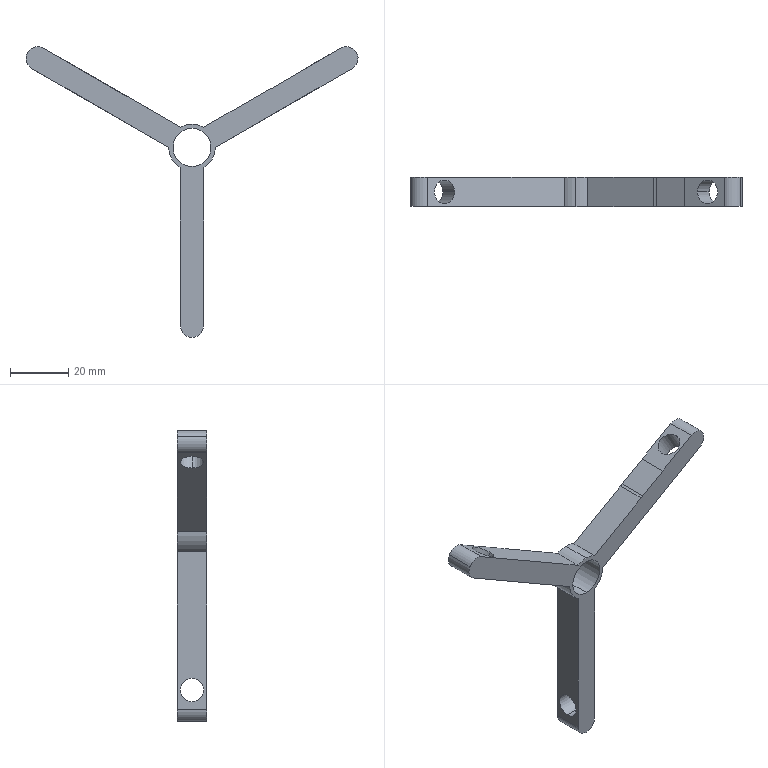Part | SolidWorks | features CirPattern 2, Fillet 2, ICE 2, Cut 1, Extrusion 1 | 1 solid | 29 faces | box 113.655 x 10 x 99.5 mm | volume 13029 mm3 | cylinder 19 | plane 10 | commonest cylinder face diameters 8 x12 16 x4 13 x2 10 x1
STEP:
#1=CARTESIAN_POINT('',(48.481,5.,32.609));
#2=VERTEX_POINT('',#1);
#3=CARTESIAN_POINT('',(41.552,5.,28.609));
#4=VERTEX_POINT('',#3);
#5=CARTESIAN_POINT('',(45.017,5.,30.609));
#6=DIRECTION('',(0.5,0.,-0.866));
#7=DIRECTION('',(-0.866,0.,-0.5));
#8=AXIS2_PLACEMENT_3D('',#5,#6,#7);
#9=CIRCLE('',#8,4.);
#10=EDGE_CURVE('',#2,#4,#9,.T.);
#11=ORIENTED_EDGE('',*,*,#10,.F.);
#12=CARTESIAN_POINT('',(52.481,5.,25.681));
#13=VERTEX_POINT('',#12);
#14=CARTESIAN_POINT('',(44.981,5.,38.671));
#15=DIRECTION('',(0.5,0.,-0.866));
#16=VECTOR('',#15,1000.);
#17=LINE('',#14,#16);
#18=EDGE_CURVE('',#2,#13,#17,.T.);
#19=ORIENTED_EDGE('',*,*,#18,.T.);
#20=CARTESIAN_POINT('',(45.552,5.,21.681));
#21=VERTEX_POINT('',#20);
#22=CARTESIAN_POINT('',(49.017,5.,23.681));
#23=DIRECTION('',(0.5,0.,-0.866));
#24=DIRECTION('',(-0.866,0.,-0.5));
#25=AXIS2_PLACEMENT_3D('',#22,#23,#24);
#26=CIRCLE('',#25,4.);
#27=EDGE_CURVE('',#13,#21,#26,.T.);
#28=ORIENTED_EDGE('',*,*,#27,.T.);
#29=CARTESIAN_POINT('',(38.052,5.,34.671));
#30=DIRECTION('',(0.5,0.,-0.866));
#31=VECTOR('',#30,1000.);
#32=LINE('',#29,#31);
#33=EDGE_CURVE('',#4,#21,#32,.T.);
#34=ORIENTED_EDGE('',*,*,#33,.F.);
#35=EDGE_LOOP('',(#11,#19,#28,#34));
#36=FACE_OUTER_BOUND('',#35,.T.);
#37=CARTESIAN_POINT('',(41.517,5.,36.671));
#38=DIRECTION('',(0.5,0.,-0.866));
#39=DIRECTION('',(-0.866,0.,-0.5));
#40=AXIS2_PLACEMENT_3D('',#37,#38,#39);
#41=CYLINDRICAL_SURFACE('',#40,4.);
#42=ADVANCED_FACE('',(#36),#41,.F.);
#43=CARTESIAN_POINT('',(-52.481,5.,25.681));
#44=VERTEX_POINT('',#43);
#45=CARTESIAN_POINT('',(-45.552,5.,21.681));
#46=VERTEX_POINT('',#45);
#47=CARTESIAN_POINT('',(-49.017,5.,23.681));
#48=DIRECTION('',(0.5,0.,0.866));
#49=DIRECTION('',(0.866,0.,-0.5));
#50=AXIS2_PLACEMENT_3D('',#47,#48,#49);
#51=CIRCLE('',#50,4.);
#52=EDGE_CURVE('',#44,#46,#51,.T.);
#53=ORIENTED_EDGE('',*,*,#52,.F.);
#54=CARTESIAN_POINT('',(-48.481,5.,32.609));
#55=VERTEX_POINT('',#54);
#56=CARTESIAN_POINT('',(-55.981,5.,19.619));
#57=DIRECTION('',(0.5,0.,0.866));
#58=VECTOR('',#57,1000.);
#59=LINE('',#56,#58);
#60=EDGE_CURVE('',#44,#55,#59,.T.);
#61=ORIENTED_EDGE('',*,*,#60,.T.);
#62=CARTESIAN_POINT('',(-41.552,5.,28.609));
#63=VERTEX_POINT('',#62);
#64=CARTESIAN_POINT('',(-45.017,5.,30.609));
#65=DIRECTION('',(0.5,0.,0.866));
#66=DIRECTION('',(0.866,0.,-0.5));
#67=AXIS2_PLACEMENT_3D('',#64,#65,#66);
#68=CIRCLE('',#67,4.);
#69=EDGE_CURVE('',#55,#63,#68,.T.);
#70=ORIENTED_EDGE('',*,*,#69,.T.);
#71=CARTESIAN_POINT('',(-49.052,5.,15.619));
#72=DIRECTION('',(0.5,0.,0.866));
#73=VECTOR('',#72,1000.);
#74=LINE('',#71,#73);
#75=EDGE_CURVE('',#46,#63,#74,.T.);
#76=ORIENTED_EDGE('',*,*,#75,.F.);
#77=EDGE_LOOP('',(#53,#61,#70,#76));
#78=FACE_OUTER_BOUND('',#77,.T.);
#79=CARTESIAN_POINT('',(-52.517,5.,17.619));
#80=DIRECTION('',(0.5,0.,0.866));
#81=DIRECTION('',(0.866,0.,-0.5));
#82=AXIS2_PLACEMENT_3D('',#79,#80,#81);
#83=CYLINDRICAL_SURFACE('',#82,4.);
#84=ADVANCED_FACE('',(#78),#83,.F.);
#85=CARTESIAN_POINT('',(4.,5.,-58.29));
#86=VERTEX_POINT('',#85);
#87=CARTESIAN_POINT('',(4.,5.,-50.29));
#88=VERTEX_POINT('',#87);
#89=CARTESIAN_POINT('',(4.,5.,-54.29));
#90=DIRECTION('',(-1.,0.,0.));
#91=DIRECTION('',(0.,0.,1.));
#92=AXIS2_PLACEMENT_3D('',#89,#90,#91);
#93=CIRCLE('',#92,4.);
#94=EDGE_CURVE('',#86,#88,#93,.T.);
#95=ORIENTED_EDGE('',*,*,#94,.F.);
#96=CARTESIAN_POINT('',(-4.,5.,-58.29));
#97=VERTEX_POINT('',#96);
#98=CARTESIAN_POINT('',(11.,5.,-58.29));
#99=DIRECTION('',(-1.,0.,0.));
#100=VECTOR('',#99,1000.);
#101=LINE('',#98,#100);
#102=EDGE_CURVE('',#86,#97,#101,.T.);
#103=ORIENTED_EDGE('',*,*,#102,.T.);
#104=CARTESIAN_POINT('',(-4.,5.,-50.29));
#105=VERTEX_POINT('',#104);
#106=CARTESIAN_POINT('',(-4.,5.,-54.29));
#107=DIRECTION('',(-1.,0.,0.));
#108=DIRECTION('',(0.,0.,1.));
#109=AXIS2_PLACEMENT_3D('',#106,#107,#108);
#110=CIRCLE('',#109,4.);
#111=EDGE_CURVE('',#97,#105,#110,.T.);
#112=ORIENTED_EDGE('',*,*,#111,.T.);
#113=CARTESIAN_POINT('',(11.,5.,-50.29));
#114=DIRECTION('',(-1.,0.,0.));
#115=VECTOR('',#114,1000.);
#116=LINE('',#113,#115);
#117=EDGE_CURVE('',#88,#105,#116,.T.);
#118=ORIENTED_EDGE('',*,*,#117,.F.);
#119=EDGE_LOOP('',(#95,#103,#112,#118));
#120=FACE_OUTER_BOUND('',#119,.T.);
#121=CARTESIAN_POINT('',(11.,5.,-54.29));
#122=DIRECTION('',(-1.,0.,0.));
#123=DIRECTION('',(0.,0.,1.));
#124=AXIS2_PLACEMENT_3D('',#121,#122,#123);
#125=CYLINDRICAL_SURFACE('',#124,4.);
#126=ADVANCED_FACE('',(#120),#125,.F.);
#127=CARTESIAN_POINT('',(0.,0.,8.));
#128=VERTEX_POINT('',#127);
#129=CARTESIAN_POINT('',(-4.,0.,6.928));
#130=VERTEX_POINT('',#129);
#131=CARTESIAN_POINT('',(0.,0.,0.));
#132=DIRECTION('',(0.,-1.,0.));
#133=DIRECTION('',(0.,0.,1.));
#134=AXIS2_PLACEMENT_3D('',#131,#132,#133);
#135=CIRCLE('',#134,8.);
#136=EDGE_CURVE('',#128,#130,#135,.T.);
#137=ORIENTED_EDGE('',*,*,#136,.F.);
#138=CARTESIAN_POINT('',(0.,10.,8.));
#139=VERTEX_POINT('',#138);
#140=CARTESIAN_POINT('',(0.,-14.,8.));
#141=DIRECTION('',(0.,1.,0.));
#142=VECTOR('',#141,1000.);
#143=LINE('',#140,#142);
#144=EDGE_CURVE('',#128,#139,#143,.T.);
#145=ORIENTED_EDGE('',*,*,#144,.T.);
#146=CARTESIAN_POINT('',(-4.,10.,6.928));
#147=VERTEX_POINT('',#146);
#148=CARTESIAN_POINT('',(0.,10.,0.));
#149=DIRECTION('',(0.,-1.,0.));
#150=DIRECTION('',(-0.866,0.,-0.5));
#151=AXIS2_PLACEMENT_3D('',#148,#149,#150);
#152=CIRCLE('',#151,8.);
#153=EDGE_CURVE('',#139,#147,#152,.T.);
#154=ORIENTED_EDGE('',*,*,#153,.T.);
#155=CARTESIAN_POINT('',(-4.,-14.,6.928));
#156=DIRECTION('',(0.,1.,0.));
#157=VECTOR('',#156,1000.);
#158=LINE('',#155,#157);
#159=EDGE_CURVE('',#130,#147,#158,.T.);
#160=ORIENTED_EDGE('',*,*,#159,.F.);
#161=EDGE_LOOP('',(#137,#145,#154,#160));
#162=FACE_OUTER_BOUND('',#161,.T.);
#163=CARTESIAN_POINT('',(0.,-14.,0.));
#164=DIRECTION('',(0.,1.,0.));
#165=DIRECTION('',(0.,0.,1.));
#166=AXIS2_PLACEMENT_3D('',#163,#164,#165);
#167=CYLINDRICAL_SURFACE('',#166,8.);
#168=ADVANCED_FACE('',(#162),#167,.T.);
#169=CARTESIAN_POINT('',(0.,10.,6.5));
#170=VERTEX_POINT('',#169);
#171=CARTESIAN_POINT('',(0.,10.,-6.5));
#172=VERTEX_POINT('',#171);
#173=CARTESIAN_POINT('',(0.,10.,0.));
#174=DIRECTION('',(0.,-1.,0.));
#175=DIRECTION('',(0.,0.,-1.));
#176=AXIS2_PLACEMENT_3D('',#173,#174,#175);
#177=CIRCLE('',#176,6.5);
#178=EDGE_CURVE('',#170,#172,#177,.T.);
#179=ORIENTED_EDGE('',*,*,#178,.F.);
#180=CARTESIAN_POINT('',(0.,0.,6.5));
#181=VERTEX_POINT('',#180);
#182=CARTESIAN_POINT('',(0.,10.,6.5));
#183=DIRECTION('',(0.,-1.,0.));
#184=VECTOR('',#183,1000.);
#185=LINE('',#182,#184);
#186=EDGE_CURVE('',#170,#181,#185,.T.);
#187=ORIENTED_EDGE('',*,*,#186,.T.);
#188=CARTESIAN_POINT('',(0.,0.,-6.5));
#189=VERTEX_POINT('',#188);
#190=CARTESIAN_POINT('',(0.,0.,0.));
#191=DIRECTION('',(0.,-1.,0.));
#192=DIRECTION('',(0.,0.,-1.));
#193=AXIS2_PLACEMENT_3D('',#190,#191,#192);
#194=CIRCLE('',#193,6.5);
#195=EDGE_CURVE('',#181,#189,#194,.T.);
#196=ORIENTED_EDGE('',*,*,#195,.T.);
#197=CARTESIAN_POINT('',(0.,10.,-6.5));
#198=DIRECTION('',(0.,-1.,0.));
#199=VECTOR('',#198,1000.);
#200=LINE('',#197,#199);
#201=EDGE_CURVE('',#172,#189,#200,.T.);
#202=ORIENTED_EDGE('',*,*,#201,.F.);
#203=EDGE_LOOP('',(#179,#187,#196,#202));
#204=FACE_OUTER_BOUND('',#203,.T.);
#205=CARTESIAN_POINT('',(0.,10.,0.));
#206=DIRECTION('',(0.,-1.,0.));
#207=DIRECTION('',(0.,0.,-1.));
#208=AXIS2_PLACEMENT_3D('',#205,#206,#207);
#209=CYLINDRICAL_SURFACE('',#208,6.5);
#210=ADVANCED_FACE('',(#204),#209,.F.);
#211=CARTESIAN_POINT('',(27.386,10.,20.333));
#212=VERTEX_POINT('',#211);
#213=CARTESIAN_POINT('',(36.971,10.,25.964));
#214=VERTEX_POINT('',#213);
#215=CARTESIAN_POINT('',(36.971,10.,25.964));
#216=DIRECTION('',(0.8622,0.,0.5066));
#217=VECTOR('',#216,1000.);
#218=LINE('',#215,#217);
#219=EDGE_CURVE('',#212,#214,#218,.T.);
#220=ORIENTED_EDGE('',*,*,#219,.F.);
#221=CARTESIAN_POINT('',(27.386,0.,20.333));
#222=VERTEX_POINT('',#221);
#223=CARTESIAN_POINT('',(27.386,0.,20.333));
#224=DIRECTION('',(0.,-1.,0.));
#225=VECTOR('',#224,1000.);
#226=LINE('',#223,#225);
#227=EDGE_CURVE('',#212,#222,#226,.T.);
#228=ORIENTED_EDGE('',*,*,#227,.T.);
#229=CARTESIAN_POINT('',(36.971,0.,25.964));
#230=VERTEX_POINT('',#229);
#231=CARTESIAN_POINT('',(36.971,0.,25.964));
#232=DIRECTION('',(0.8622,0.,0.5066));
#233=VECTOR('',#232,1000.);
#234=LINE('',#231,#233);
#235=EDGE_CURVE('',#222,#230,#234,.T.);
#236=ORIENTED_EDGE('',*,*,#235,.T.);
#237=CARTESIAN_POINT('',(36.971,10.,25.964));
#238=DIRECTION('',(0.,-1.,0.));
#239=VECTOR('',#238,1000.);
#240=LINE('',#237,#239);
#241=EDGE_CURVE('',#214,#230,#240,.T.);
#242=ORIENTED_EDGE('',*,*,#241,.F.);
#243=EDGE_LOOP('',(#220,#228,#236,#242));
#244=FACE_OUTER_BOUND('',#243,.T.);
#245=CARTESIAN_POINT('',(36.971,10.,25.964));
#246=DIRECTION('',(0.5066,0.,-0.8622));
#247=DIRECTION('',(-0.8622,0.,-0.5066));
#248=AXIS2_PLACEMENT_3D('',#245,#246,#247);
#249=PLANE('',#248);
#250=ADVANCED_FACE('',(#244),#249,.F.);
#251=CARTESIAN_POINT('',(45.017,5.,30.609));
#252=DIRECTION('',(0.5,0.,-0.866));
#253=DIRECTION('',(-0.866,0.,-0.5));
#254=AXIS2_PLACEMENT_3D('',#251,#252,#253);
#255=CIRCLE('',#254,4.);
#256=EDGE_CURVE('',#4,#2,#255,.T.);
#257=ORIENTED_EDGE('',*,*,#256,.T.);
#258=ORIENTED_EDGE('',*,*,#10,.T.);
#259=EDGE_LOOP('',(#257,#258));
#260=FACE_BOUND('',#259,.T.);
#261=CARTESIAN_POINT('',(50.828,0.,33.964));
#262=VERTEX_POINT('',#261);
#263=CARTESIAN_POINT('',(54.292,0.,35.964));
#264=DIRECTION('',(0.866,0.,0.5));
#265=VECTOR('',#264,1000.);
#266=LINE('',#263,#265);
#267=EDGE_CURVE('',#230,#262,#266,.T.);
#268=ORIENTED_EDGE('',*,*,#267,.T.);
#269=CARTESIAN_POINT('',(50.828,10.,33.964));
#270=VERTEX_POINT('',#269);
#271=CARTESIAN_POINT('',(50.828,10.,33.964));
#272=DIRECTION('',(0.,1.,0.));
#273=VECTOR('',#272,1000.);
#274=LINE('',#271,#273);
#275=EDGE_CURVE('',#262,#270,#274,.T.);
#276=ORIENTED_EDGE('',*,*,#275,.T.);
#277=CARTESIAN_POINT('',(54.292,10.,35.964));
#278=DIRECTION('',(0.866,0.,0.5));
#279=VECTOR('',#278,1000.);
#280=LINE('',#277,#279);
#281=EDGE_CURVE('',#214,#270,#280,.T.);
#282=ORIENTED_EDGE('',*,*,#281,.F.);
#283=ORIENTED_EDGE('',*,*,#241,.T.);
#284=EDGE_LOOP('',(#268,#276,#282,#283));
#285=FACE_OUTER_BOUND('',#284,.T.);
#286=CARTESIAN_POINT('',(54.292,10.,35.964));
#287=DIRECTION('',(0.5,0.,-0.866));
#288=DIRECTION('',(-0.866,0.,-0.5));
#289=AXIS2_PLACEMENT_3D('',#286,#287,#288);
#290=PLANE('',#289);
#291=ADVANCED_FACE('',(#260,#285),#290,.F.);
#292=CARTESIAN_POINT('',(49.017,5.,23.681));
#293=DIRECTION('',(0.5,0.,-0.866));
#294=DIRECTION('',(-0.866,0.,-0.5));
#295=AXIS2_PLACEMENT_3D('',#292,#293,#294);
#296=CIRCLE('',#295,4.);
#297=EDGE_CURVE('',#21,#13,#296,.T.);
#298=ORIENTED_EDGE('',*,*,#297,.F.);
#299=ORIENTED_EDGE('',*,*,#27,.F.);
#300=EDGE_LOOP('',(#298,#299));
#301=FACE_BOUND('',#300,.T.);
#302=CARTESIAN_POINT('',(54.828,0.,27.036));
#303=VERTEX_POINT('',#302);
#304=CARTESIAN_POINT('',(8.,0.,0.));
#305=VERTEX_POINT('',#304);
#306=CARTESIAN_POINT('',(40.971,0.,19.036));
#307=DIRECTION('',(-0.866,0.,-0.5));
#308=VECTOR('',#307,1000.);
#309=LINE('',#306,#308);
#310=EDGE_CURVE('',#303,#305,#309,.T.);
#311=ORIENTED_EDGE('',*,*,#310,.T.);
#312=CARTESIAN_POINT('',(8.,10.,0.));
#313=VERTEX_POINT('',#312);
#314=CARTESIAN_POINT('',(8.,-14.,0.));
#315=DIRECTION('',(0.,1.,0.));
#316=VECTOR('',#315,1000.);
#317=LINE('',#314,#316);
#318=EDGE_CURVE('',#305,#313,#317,.T.);
#319=ORIENTED_EDGE('',*,*,#318,.T.);
#320=CARTESIAN_POINT('',(54.828,10.,27.036));
#321=VERTEX_POINT('',#320);
#322=CARTESIAN_POINT('',(58.292,10.,29.036));
#323=DIRECTION('',(-0.866,0.,-0.5));
#324=VECTOR('',#323,1000.);
#325=LINE('',#322,#324);
#326=EDGE_CURVE('',#321,#313,#325,.T.);
#327=ORIENTED_EDGE('',*,*,#326,.F.);
#328=CARTESIAN_POINT('',(54.828,10.,27.036));
#329=DIRECTION('',(0.,-1.,0.));
#330=VECTOR('',#329,1000.);
#331=LINE('',#328,#330);
#332=EDGE_CURVE('',#321,#303,#331,.T.);
#333=ORIENTED_EDGE('',*,*,#332,.T.);
#334=EDGE_LOOP('',(#311,#319,#327,#333));
#335=FACE_OUTER_BOUND('',#334,.T.);
#336=CARTESIAN_POINT('',(40.971,10.,19.036));
#337=DIRECTION('',(-0.5,0.,0.866));
#338=DIRECTION('',(0.866,0.,0.5));
#339=AXIS2_PLACEMENT_3D('',#336,#337,#338);
#340=PLANE('',#339);
#341=ADVANCED_FACE('',(#301,#335),#340,.F.);
#342=CARTESIAN_POINT('',(4.,5.,-54.29));
#343=DIRECTION('',(-1.,0.,0.));
#344=DIRECTION('',(0.,0.,1.));
#345=AXIS2_PLACEMENT_3D('',#342,#343,#344);
#346=CIRCLE('',#345,4.);
#347=EDGE_CURVE('',#88,#86,#346,.T.);
#348=ORIENTED_EDGE('',*,*,#347,.T.);
#349=ORIENTED_EDGE('',*,*,#94,.T.);
#350=EDGE_LOOP('',(#348,#349));
#351=FACE_BOUND('',#350,.T.);
#352=CARTESIAN_POINT('',(4.,10.,-6.928));
#353=VERTEX_POINT('',#352);
#354=CARTESIAN_POINT('',(4.,10.,-61.));
#355=VERTEX_POINT('',#354);
#356=CARTESIAN_POINT('',(4.,10.,-45.));
#357=DIRECTION('',(0.,0.,-1.));
#358=VECTOR('',#357,1000.);
#359=LINE('',#356,#358);
#360=EDGE_CURVE('',#353,#355,#359,.T.);
#361=ORIENTED_EDGE('',*,*,#360,.F.);
#362=CARTESIAN_POINT('',(4.,0.,-6.928));
#363=VERTEX_POINT('',#362);
#364=CARTESIAN_POINT('',(4.,-14.,-6.928));
#365=DIRECTION('',(0.,1.,0.));
#366=VECTOR('',#365,1000.);
#367=LINE('',#364,#366);
#368=EDGE_CURVE('',#363,#353,#367,.T.);
#369=ORIENTED_EDGE('',*,*,#368,.F.);
#370=CARTESIAN_POINT('',(4.,0.,-61.));
#371=VERTEX_POINT('',#370);
#372=CARTESIAN_POINT('',(4.,0.,-65.));
#373=DIRECTION('',(0.,0.,-1.));
#374=VECTOR('',#373,1000.);
#375=LINE('',#372,#374);
#376=EDGE_CURVE('',#363,#371,#375,.T.);
#377=ORIENTED_EDGE('',*,*,#376,.T.);
#378=CARTESIAN_POINT('',(4.,10.,-61.));
#379=DIRECTION('',(0.,1.,0.));
#380=VECTOR('',#379,1000.);
#381=LINE('',#378,#380);
#382=EDGE_CURVE('',#371,#355,#381,.T.);
#383=ORIENTED_EDGE('',*,*,#382,.T.);
#384=EDGE_LOOP('',(#361,#369,#377,#383));
#385=FACE_OUTER_BOUND('',#384,.T.);
#386=CARTESIAN_POINT('',(4.,10.,-65.));
#387=DIRECTION('',(-1.,0.,0.));
#388=DIRECTION('',(0.,0.,1.));
#389=AXIS2_PLACEMENT_3D('',#386,#387,#388);
#390=PLANE('',#389);
#391=ADVANCED_FACE('',(#351,#385),#390,.F.);
#392=CARTESIAN_POINT('',(-4.,5.,-54.29));
#393=DIRECTION('',(-1.,0.,0.));
#394=DIRECTION('',(0.,0.,1.));
#395=AXIS2_PLACEMENT_3D('',#392,#393,#394);
#396=CIRCLE('',#395,4.);
#397=EDGE_CURVE('',#105,#97,#396,.T.);
#398=ORIENTED_EDGE('',*,*,#397,.F.);
#399=ORIENTED_EDGE('',*,*,#111,.F.);
#400=EDGE_LOOP('',(#398,#399));
#401=FACE_BOUND('',#400,.T.);
#402=CARTESIAN_POINT('',(-4.,0.,-61.));
#403=VERTEX_POINT('',#402);
#404=CARTESIAN_POINT('',(-4.,0.,-6.928));
#405=VERTEX_POINT('',#404);
#406=CARTESIAN_POINT('',(-4.,0.,-45.));
#407=DIRECTION('',(0.,0.,1.));
#408=VECTOR('',#407,1000.);
#409=LINE('',#406,#408);
#410=EDGE_CURVE('',#403,#405,#409,.T.);
#411=ORIENTED_EDGE('',*,*,#410,.T.);
#412=CARTESIAN_POINT('',(-4.,10.,-6.928));
#413=VERTEX_POINT('',#412);
#414=CARTESIAN_POINT('',(-4.,-14.,-6.928));
#415=DIRECTION('',(0.,1.,0.));
#416=VECTOR('',#415,1000.);
#417=LINE('',#414,#416);
#418=EDGE_CURVE('',#405,#413,#417,.T.);
#419=ORIENTED_EDGE('',*,*,#418,.T.);
#420=CARTESIAN_POINT('',(-4.,10.,-61.));
#421=VERTEX_POINT('',#420);
#422=CARTESIAN_POINT('',(-4.,10.,-65.));
#423=DIRECTION('',(0.,0.,1.));
#424=VECTOR('',#423,1000.);
#425=LINE('',#422,#424);
#426=EDGE_CURVE('',#421,#413,#425,.T.);
#427=ORIENTED_EDGE('',*,*,#426,.F.);
#428=CARTESIAN_POINT('',(-4.,10.,-61.));
#429=DIRECTION('',(0.,-1.,0.));
#430=VECTOR('',#429,1000.);
#431=LINE('',#428,#430);
#432=EDGE_CURVE('',#421,#403,#431,.T.);
#433=ORIENTED_EDGE('',*,*,#432,.T.);
#434=EDGE_LOOP('',(#411,#419,#427,#433));
#435=FACE_OUTER_BOUND('',#434,.T.);
#436=CARTESIAN_POINT('',(-4.,10.,-45.));
#437=DIRECTION('',(1.,0.,0.));
#438=DIRECTION('',(0.,0.,-1.));
#439=AXIS2_PLACEMENT_3D('',#436,#437,#438);
#440=PLANE('',#439);
#441=ADVANCED_FACE('',(#401,#435),#440,.F.);
#442=CARTESIAN_POINT('',(-49.017,5.,23.681));
#443=DIRECTION('',(0.5,0.,0.866));
#444=DIRECTION('',(0.866,0.,-0.5));
#445=AXIS2_PLACEMENT_3D('',#442,#443,#444);
#446=CIRCLE('',#445,4.);
#447=EDGE_CURVE('',#46,#44,#446,.T.);
#448=ORIENTED_EDGE('',*,*,#447,.T.);
#449=ORIENTED_EDGE('',*,*,#52,.T.);
#450=EDGE_LOOP('',(#448,#449));
#451=FACE_BOUND('',#450,.T.);
#452=CARTESIAN_POINT('',(-8.,10.,0.));
#453=VERTEX_POINT('',#452);
#454=CARTESIAN_POINT('',(-54.828,10.,27.036));
#455=VERTEX_POINT('',#454);
#456=CARTESIAN_POINT('',(-40.971,10.,19.036));
#457=DIRECTION('',(-0.866,0.,0.5));
#458=VECTOR('',#457,1000.);
#459=LINE('',#456,#458);
#460=EDGE_CURVE('',#453,#455,#459,.T.);
#461=ORIENTED_EDGE('',*,*,#460,.F.);
#462=CARTESIAN_POINT('',(-8.,0.,0.));
#463=VERTEX_POINT('',#462);
#464=CARTESIAN_POINT('',(-8.,-14.,0.));
#465=DIRECTION('',(0.,1.,0.));
#466=VECTOR('',#465,1000.);
#467=LINE('',#464,#466);
#468=EDGE_CURVE('',#463,#453,#467,.T.);
#469=ORIENTED_EDGE('',*,*,#468,.F.);
#470=CARTESIAN_POINT('',(-54.828,0.,27.036));
#471=VERTEX_POINT('',#470);
#472=CARTESIAN_POINT('',(-58.292,0.,29.036));
#473=DIRECTION('',(-0.866,0.,0.5));
#474=VECTOR('',#473,1000.);
#475=LINE('',#472,#474);
#476=EDGE_CURVE('',#463,#471,#475,.T.);
#477=ORIENTED_EDGE('',*,*,#476,.T.);
#478=CARTESIAN_POINT('',(-54.828,10.,27.036));
#479=DIRECTION('',(0.,1.,0.));
#480=VECTOR('',#479,1000.);
#481=LINE('',#478,#480);
#482=EDGE_CURVE('',#471,#455,#481,.T.);
#483=ORIENTED_EDGE('',*,*,#482,.T.);
#484=EDGE_LOOP('',(#461,#469,#477,#483));
#485=FACE_OUTER_BOUND('',#484,.T.);
#486=CARTESIAN_POINT('',(-58.292,10.,29.036));
#487=DIRECTION('',(0.5,0.,0.866));
#488=DIRECTION('',(0.866,0.,-0.5));
#489=AXIS2_PLACEMENT_3D('',#486,#487,#488);
#490=PLANE('',#489);
#491=ADVANCED_FACE('',(#451,#485),#490,.F.);
#492=CARTESIAN_POINT('',(-45.017,5.,30.609));
#493=DIRECTION('',(0.5,0.,0.866));
#494=DIRECTION('',(0.866,0.,-0.5));
#495=AXIS2_PLACEMENT_3D('',#492,#493,#494);
#496=CIRCLE('',#495,4.);
#497=EDGE_CURVE('',#63,#55,#496,.T.);
#498=ORIENTED_EDGE('',*,*,#497,.F.);
#499=ORIENTED_EDGE('',*,*,#69,.F.);
#500=EDGE_LOOP('',(#498,#499));
#501=FACE_BOUND('',#500,.T.);
#502=CARTESIAN_POINT('',(-50.828,0.,33.964));
#503=VERTEX_POINT('',#502);
#504=CARTESIAN_POINT('',(-36.971,0.,25.964));
#505=DIRECTION('',(0.866,0.,-0.5));
#506=VECTOR('',#505,1000.);
#507=LINE('',#504,#506);
#508=EDGE_CURVE('',#503,#130,#507,.T.);
#509=ORIENTED_EDGE('',*,*,#508,.T.);
#510=ORIENTED_EDGE('',*,*,#159,.T.);
#511=CARTESIAN_POINT('',(-50.828,10.,33.964));
#512=VERTEX_POINT('',#511);
#513=CARTESIAN_POINT('',(-54.292,10.,35.964));
#514=DIRECTION('',(0.866,0.,-0.5));
#515=VECTOR('',#514,1000.);
#516=LINE('',#513,#515);
#517=EDGE_CURVE('',#512,#147,#516,.T.);
#518=ORIENTED_EDGE('',*,*,#517,.F.);
#519=CARTESIAN_POINT('',(-50.828,10.,33.964));
#520=DIRECTION('',(0.,-1.,0.));
#521=VECTOR('',#520,1000.);
#522=LINE('',#519,#521);
#523=EDGE_CURVE('',#512,#503,#522,.T.);
#524=ORIENTED_EDGE('',*,*,#523,.T.);
#525=EDGE_LOOP('',(#509,#510,#518,#524));
#526=FACE_OUTER_BOUND('',#525,.T.);
#527=CARTESIAN_POINT('',(-36.971,10.,25.964));
#528=DIRECTION('',(-0.5,0.,-0.866));
#529=DIRECTION('',(-0.866,0.,0.5));
#530=AXIS2_PLACEMENT_3D('',#527,#528,#529);
#531=PLANE('',#530);
#532=ADVANCED_FACE('',(#501,#526),#531,.F.);
#533=ORIENTED_EDGE('',*,*,#426,.T.);
#534=CARTESIAN_POINT('',(0.,10.,0.));
#535=DIRECTION('',(0.,-1.,0.));
#536=DIRECTION('',(0.866,0.,-0.5));
#537=AXIS2_PLACEMENT_3D('',#534,#535,#536);
#538=CIRCLE('',#537,8.);
#539=EDGE_CURVE('',#453,#413,#538,.T.);
#540=ORIENTED_EDGE('',*,*,#539,.F.);
#541=ORIENTED_EDGE('',*,*,#460,.T.);
#542=CARTESIAN_POINT('',(-56.292,10.,32.5));
#543=VERTEX_POINT('',#542);
#544=CARTESIAN_POINT('',(-52.828,10.,30.5));
#545=DIRECTION('',(0.,1.,0.));
#546=DIRECTION('',(0.,0.,1.));
#547=AXIS2_PLACEMENT_3D('',#544,#545,#546);
#548=CIRCLE('',#547,4.);
#549=EDGE_CURVE('',#455,#543,#548,.T.);
#550=ORIENTED_EDGE('',*,*,#549,.T.);
#551=CARTESIAN_POINT('',(-52.828,10.,30.5));
#552=DIRECTION('',(0.,1.,0.));
#553=DIRECTION('',(0.,0.,1.));
#554=AXIS2_PLACEMENT_3D('',#551,#552,#553);
#555=CIRCLE('',#554,4.);
#556=EDGE_CURVE('',#543,#512,#555,.T.);
#557=ORIENTED_EDGE('',*,*,#556,.T.);
#558=ORIENTED_EDGE('',*,*,#517,.T.);
#559=ORIENTED_EDGE('',*,*,#153,.F.);
#560=CARTESIAN_POINT('',(4.,10.,6.928));
#561=VERTEX_POINT('',#560);
#562=CARTESIAN_POINT('',(0.,10.,0.));
#563=DIRECTION('',(0.,-1.,0.));
#564=DIRECTION('',(-0.866,0.,-0.5));
#565=AXIS2_PLACEMENT_3D('',#562,#563,#564);
#566=CIRCLE('',#565,8.);
#567=EDGE_CURVE('',#561,#139,#566,.T.);
#568=ORIENTED_EDGE('',*,*,#567,.F.);
#569=CARTESIAN_POINT('',(26.517,10.,19.928));
#570=VERTEX_POINT('',#569);
#571=CARTESIAN_POINT('',(27.292,10.,20.376));
#572=DIRECTION('',(-0.866,0.,-0.5));
#573=VECTOR('',#572,1000.);
#574=LINE('',#571,#573);
#575=EDGE_CURVE('',#570,#561,#574,.T.);
#576=ORIENTED_EDGE('',*,*,#575,.F.);
#577=CARTESIAN_POINT('',(24.853,10.,24.644));
#578=DIRECTION('',(0.,-1.,0.));
#579=DIRECTION('',(0.,0.,1.));
#580=AXIS2_PLACEMENT_3D('',#577,#578,#579);
#581=CIRCLE('',#580,5.);
#582=EDGE_CURVE('',#570,#212,#581,.T.);
#583=ORIENTED_EDGE('',*,*,#582,.T.);
#584=ORIENTED_EDGE('',*,*,#219,.T.);
#585=ORIENTED_EDGE('',*,*,#281,.T.);
#586=CARTESIAN_POINT('',(56.292,10.,32.5));
#587=VERTEX_POINT('',#586);
#588=CARTESIAN_POINT('',(52.828,10.,30.5));
#589=DIRECTION('',(0.,1.,0.));
#590=DIRECTION('',(0.,0.,1.));
#591=AXIS2_PLACEMENT_3D('',#588,#589,#590);
#592=CIRCLE('',#591,4.);
#593=EDGE_CURVE('',#270,#587,#592,.T.);
#594=ORIENTED_EDGE('',*,*,#593,.T.);
#595=CARTESIAN_POINT('',(52.828,10.,30.5));
#596=DIRECTION('',(0.,1.,0.));
#597=DIRECTION('',(0.,0.,1.));
#598=AXIS2_PLACEMENT_3D('',#595,#596,#597);
#599=CIRCLE('',#598,4.);
#600=EDGE_CURVE('',#587,#321,#599,.T.);
#601=ORIENTED_EDGE('',*,*,#600,.T.);
#602=ORIENTED_EDGE('',*,*,#326,.T.);
#603=CARTESIAN_POINT('',(0.,10.,0.));
#604=DIRECTION('',(0.,-1.,0.));
#605=DIRECTION('',(0.,0.,1.));
#606=AXIS2_PLACEMENT_3D('',#603,#604,#605);
#607=CIRCLE('',#606,8.);
#608=EDGE_CURVE('',#353,#313,#607,.T.);
#609=ORIENTED_EDGE('',*,*,#608,.F.);
#610=ORIENTED_EDGE('',*,*,#360,.T.);
#611=CARTESIAN_POINT('',(0.,10.,-65.));
#612=VERTEX_POINT('',#611);
#613=CARTESIAN_POINT('',(0.,10.,-61.));
#614=DIRECTION('',(0.,1.,0.));
#615=DIRECTION('',(0.,0.,1.));
#616=AXIS2_PLACEMENT_3D('',#613,#614,#615);
#617=CIRCLE('',#616,4.);
#618=EDGE_CURVE('',#355,#612,#617,.T.);
#619=ORIENTED_EDGE('',*,*,#618,.T.);
#620=CARTESIAN_POINT('',(0.,10.,-61.));
#621=DIRECTION('',(0.,1.,0.));
#622=DIRECTION('',(0.,0.,1.));
#623=AXIS2_PLACEMENT_3D('',#620,#621,#622);
#624=CIRCLE('',#623,4.);
#625=EDGE_CURVE('',#612,#421,#624,.T.);
#626=ORIENTED_EDGE('',*,*,#625,.T.);
#627=EDGE_LOOP('',(#533,#540,#541,#550,#557,#558,#559,#568,#576,#583,#584,#585,#594,#601,#602,#609,#610,#619,#626));
#628=FACE_OUTER_BOUND('',#627,.T.);
#629=CARTESIAN_POINT('',(0.,10.,0.));
#630=DIRECTION('',(0.,-1.,0.));
#631=DIRECTION('',(0.,0.,-1.));
#632=AXIS2_PLACEMENT_3D('',#629,#630,#631);
#633=CIRCLE('',#632,6.5);
#634=EDGE_CURVE('',#172,#170,#633,.T.);
#635=ORIENTED_EDGE('',*,*,#634,.T.);
#636=ORIENTED_EDGE('',*,*,#178,.T.);
#637=EDGE_LOOP('',(#635,#636));
#638=FACE_BOUND('',#637,.T.);
#639=CARTESIAN_POINT('',(0.,10.,0.));
#640=DIRECTION('',(0.,1.,0.));
#641=DIRECTION('',(0.,0.,1.));
#642=AXIS2_PLACEMENT_3D('',#639,#640,#641);
#643=PLANE('',#642);
#644=ADVANCED_FACE('',(#628,#638),#643,.T.);
#645=CARTESIAN_POINT('',(0.,0.,0.));
#646=DIRECTION('',(0.,-1.,0.));
#647=DIRECTION('',(0.,0.,-1.));
#648=AXIS2_PLACEMENT_3D('',#645,#646,#647);
#649=CIRCLE('',#648,6.5);
#650=EDGE_CURVE('',#189,#181,#649,.T.);
#651=ORIENTED_EDGE('',*,*,#650,.F.);
#652=ORIENTED_EDGE('',*,*,#195,.F.);
#653=EDGE_LOOP('',(#651,#652));
#654=FACE_BOUND('',#653,.T.);
#655=CARTESIAN_POINT('',(0.,0.,0.));
#656=DIRECTION('',(0.,-1.,0.));
#657=DIRECTION('',(0.,0.,1.));
#658=AXIS2_PLACEMENT_3D('',#655,#656,#657);
#659=CIRCLE('',#658,8.);
#660=EDGE_CURVE('',#463,#405,#659,.T.);
#661=ORIENTED_EDGE('',*,*,#660,.T.);
#662=ORIENTED_EDGE('',*,*,#410,.F.);
#663=CARTESIAN_POINT('',(0.,0.,-65.));
#664=VERTEX_POINT('',#663);
#665=CARTESIAN_POINT('',(0.,0.,-61.));
#666=DIRECTION('',(0.,-1.,0.));
#667=DIRECTION('',(0.,0.,1.));
#668=AXIS2_PLACEMENT_3D('',#665,#666,#667);
#669=CIRCLE('',#668,4.);
#670=EDGE_CURVE('',#403,#664,#669,.T.);
#671=ORIENTED_EDGE('',*,*,#670,.T.);
#672=CARTESIAN_POINT('',(0.,0.,-61.));
#673=DIRECTION('',(0.,-1.,0.));
#674=DIRECTION('',(0.,0.,1.));
#675=AXIS2_PLACEMENT_3D('',#672,#673,#674);
#676=CIRCLE('',#675,4.);
#677=EDGE_CURVE('',#664,#371,#676,.T.);
#678=ORIENTED_EDGE('',*,*,#677,.T.);
#679=ORIENTED_EDGE('',*,*,#376,.F.);
#680=CARTESIAN_POINT('',(0.,0.,0.));
#681=DIRECTION('',(0.,-1.,0.));
#682=DIRECTION('',(0.,0.,1.));
#683=AXIS2_PLACEMENT_3D('',#680,#681,#682);
#684=CIRCLE('',#683,8.);
#685=EDGE_CURVE('',#363,#305,#684,.T.);
#686=ORIENTED_EDGE('',*,*,#685,.T.);
#687=ORIENTED_EDGE('',*,*,#310,.F.);
#688=CARTESIAN_POINT('',(56.292,0.,32.5));
#689=VERTEX_POINT('',#688);
#690=CARTESIAN_POINT('',(52.828,0.,30.5));
#691=DIRECTION('',(0.,-1.,0.));
#692=DIRECTION('',(0.,0.,1.));
#693=AXIS2_PLACEMENT_3D('',#690,#691,#692);
#694=CIRCLE('',#693,4.);
#695=EDGE_CURVE('',#303,#689,#694,.T.);
#696=ORIENTED_EDGE('',*,*,#695,.T.);
#697=CARTESIAN_POINT('',(52.828,0.,30.5));
#698=DIRECTION('',(0.,-1.,0.));
#699=DIRECTION('',(0.,0.,1.));
#700=AXIS2_PLACEMENT_3D('',#697,#698,#699);
#701=CIRCLE('',#700,4.);
#702=EDGE_CURVE('',#689,#262,#701,.T.);
#703=ORIENTED_EDGE('',*,*,#702,.T.);
#704=ORIENTED_EDGE('',*,*,#267,.F.);
#705=ORIENTED_EDGE('',*,*,#235,.F.);
#706=CARTESIAN_POINT('',(26.517,0.,19.928));
#707=VERTEX_POINT('',#706);
#708=CARTESIAN_POINT('',(24.853,0.,24.644));
#709=DIRECTION('',(0.,1.,0.));
#710=DIRECTION('',(0.,0.,1.));
#711=AXIS2_PLACEMENT_3D('',#708,#709,#710);
#712=CIRCLE('',#711,5.);
#713=EDGE_CURVE('',#222,#707,#712,.T.);
#714=ORIENTED_EDGE('',*,*,#713,.T.);
#715=CARTESIAN_POINT('',(4.,0.,6.928));
#716=VERTEX_POINT('',#715);
#717=CARTESIAN_POINT('',(-2.,0.,3.464));
#718=DIRECTION('',(-0.866,0.,-0.5));
#719=VECTOR('',#718,1000.);
#720=LINE('',#717,#719);
#721=EDGE_CURVE('',#707,#716,#720,.T.);
#722=ORIENTED_EDGE('',*,*,#721,.T.);
#723=CARTESIAN_POINT('',(0.,0.,0.));
#724=DIRECTION('',(0.,-1.,0.));
#725=DIRECTION('',(0.,0.,1.));
#726=AXIS2_PLACEMENT_3D('',#723,#724,#725);
#727=CIRCLE('',#726,8.);
#728=EDGE_CURVE('',#716,#128,#727,.T.);
#729=ORIENTED_EDGE('',*,*,#728,.T.);
#730=ORIENTED_EDGE('',*,*,#136,.T.);
#731=ORIENTED_EDGE('',*,*,#508,.F.);
#732=CARTESIAN_POINT('',(-56.292,0.,32.5));
#733=VERTEX_POINT('',#732);
#734=CARTESIAN_POINT('',(-52.828,0.,30.5));
#735=DIRECTION('',(0.,-1.,0.));
#736=DIRECTION('',(0.,0.,1.));
#737=AXIS2_PLACEMENT_3D('',#734,#735,#736);
#738=CIRCLE('',#737,4.);
#739=EDGE_CURVE('',#503,#733,#738,.T.);
#740=ORIENTED_EDGE('',*,*,#739,.T.);
#741=CARTESIAN_POINT('',(-52.828,0.,30.5));
#742=DIRECTION('',(0.,-1.,0.));
#743=DIRECTION('',(0.,0.,1.));
#744=AXIS2_PLACEMENT_3D('',#741,#742,#743);
#745=CIRCLE('',#744,4.);
#746=EDGE_CURVE('',#733,#471,#745,.T.);
#747=ORIENTED_EDGE('',*,*,#746,.T.);
#748=ORIENTED_EDGE('',*,*,#476,.F.);
#749=EDGE_LOOP('',(#661,#662,#671,#678,#679,#686,#687,#696,#703,#704,#705,#714,#722,#729,#730,#731,#740,#747,#748));
#750=FACE_OUTER_BOUND('',#749,.T.);
#751=CARTESIAN_POINT('',(0.,0.,0.));
#752=DIRECTION('',(0.,1.,0.));
#753=DIRECTION('',(0.,0.,1.));
#754=AXIS2_PLACEMENT_3D('',#751,#752,#753);
#755=PLANE('',#754);
#756=ADVANCED_FACE('',(#654,#750),#755,.F.);
#757=CARTESIAN_POINT('',(56.292,10.,32.5));
#758=DIRECTION('',(0.,-1.,0.));
#759=VECTOR('',#758,1000.);
#760=LINE('',#757,#759);
#761=EDGE_CURVE('',#587,#689,#760,.T.);
#762=ORIENTED_EDGE('',*,*,#761,.F.);
#763=ORIENTED_EDGE('',*,*,#593,.F.);
#764=ORIENTED_EDGE('',*,*,#275,.F.);
#765=ORIENTED_EDGE('',*,*,#702,.F.);
#766=EDGE_LOOP('',(#762,#763,#764,#765));
#767=FACE_OUTER_BOUND('',#766,.T.);
#768=CARTESIAN_POINT('',(52.828,10.,30.5));
#769=DIRECTION('',(0.,-1.,0.));
#770=DIRECTION('',(0.,0.,-1.));
#771=AXIS2_PLACEMENT_3D('',#768,#769,#770);
#772=CYLINDRICAL_SURFACE('',#771,4.);
#773=ADVANCED_FACE('',(#767),#772,.T.);
#774=ORIENTED_EDGE('',*,*,#600,.F.);
#775=ORIENTED_EDGE('',*,*,#761,.T.);
#776=ORIENTED_EDGE('',*,*,#695,.F.);
#777=ORIENTED_EDGE('',*,*,#332,.F.);
#778=EDGE_LOOP('',(#774,#775,#776,#777));
#779=FACE_OUTER_BOUND('',#778,.T.);
#780=CARTESIAN_POINT('',(52.828,10.,30.5));
#781=DIRECTION('',(0.,-1.,0.));
#782=DIRECTION('',(0.,0.,-1.));
#783=AXIS2_PLACEMENT_3D('',#780,#781,#782);
#784=CYLINDRICAL_SURFACE('',#783,4.);
#785=ADVANCED_FACE('',(#779),#784,.T.);
#786=CARTESIAN_POINT('',(-56.292,10.,32.5));
#787=DIRECTION('',(0.,-1.,0.));
#788=VECTOR('',#787,1000.);
#789=LINE('',#786,#788);
#790=EDGE_CURVE('',#543,#733,#789,.T.);
#791=ORIENTED_EDGE('',*,*,#790,.F.);
#792=ORIENTED_EDGE('',*,*,#549,.F.);
#793=ORIENTED_EDGE('',*,*,#482,.F.);
#794=ORIENTED_EDGE('',*,*,#746,.F.);
#795=EDGE_LOOP('',(#791,#792,#793,#794));
#796=FACE_OUTER_BOUND('',#795,.T.);
#797=CARTESIAN_POINT('',(-52.828,10.,30.5));
#798=DIRECTION('',(0.,-1.,0.));
#799=DIRECTION('',(0.,0.,-1.));
#800=AXIS2_PLACEMENT_3D('',#797,#798,#799);
#801=CYLINDRICAL_SURFACE('',#800,4.);
#802=ADVANCED_FACE('',(#796),#801,.T.);
#803=ORIENTED_EDGE('',*,*,#556,.F.);
#804=ORIENTED_EDGE('',*,*,#790,.T.);
#805=ORIENTED_EDGE('',*,*,#739,.F.);
#806=ORIENTED_EDGE('',*,*,#523,.F.);
#807=EDGE_LOOP('',(#803,#804,#805,#806));
#808=FACE_OUTER_BOUND('',#807,.T.);
#809=CARTESIAN_POINT('',(-52.828,10.,30.5));
#810=DIRECTION('',(0.,-1.,0.));
#811=DIRECTION('',(0.,0.,-1.));
#812=AXIS2_PLACEMENT_3D('',#809,#810,#811);
#813=CYLINDRICAL_SURFACE('',#812,4.);
#814=ADVANCED_FACE('',(#808),#813,.T.);
#815=ORIENTED_EDGE('',*,*,#432,.F.);
#816=ORIENTED_EDGE('',*,*,#625,.F.);
#817=CARTESIAN_POINT('',(0.,10.,-65.));
#818=DIRECTION('',(0.,1.,0.));
#819=VECTOR('',#818,1000.);
#820=LINE('',#817,#819);
#821=EDGE_CURVE('',#664,#612,#820,.T.);
#822=ORIENTED_EDGE('',*,*,#821,.F.);
#823=ORIENTED_EDGE('',*,*,#670,.F.);
#824=EDGE_LOOP('',(#815,#816,#822,#823));
#825=FACE_OUTER_BOUND('',#824,.T.);
#826=CARTESIAN_POINT('',(0.,10.,-61.));
#827=DIRECTION('',(0.,-1.,0.));
#828=DIRECTION('',(0.,0.,-1.));
#829=AXIS2_PLACEMENT_3D('',#826,#827,#828);
#830=CYLINDRICAL_SURFACE('',#829,4.);
#831=ADVANCED_FACE('',(#825),#830,.T.);
#832=ORIENTED_EDGE('',*,*,#618,.F.);
#833=ORIENTED_EDGE('',*,*,#382,.F.);
#834=ORIENTED_EDGE('',*,*,#677,.F.);
#835=ORIENTED_EDGE('',*,*,#821,.T.);
#836=EDGE_LOOP('',(#832,#833,#834,#835));
#837=FACE_OUTER_BOUND('',#836,.T.);
#838=CARTESIAN_POINT('',(0.,10.,-61.));
#839=DIRECTION('',(0.,-1.,0.));
#840=DIRECTION('',(0.,0.,-1.));
#841=AXIS2_PLACEMENT_3D('',#838,#839,#840);
#842=CYLINDRICAL_SURFACE('',#841,4.);
#843=ADVANCED_FACE('',(#837),#842,.T.);
#844=ORIENTED_EDGE('',*,*,#582,.F.);
#845=CARTESIAN_POINT('',(26.517,10.,19.928));
#846=DIRECTION('',(0.,-1.,0.));
#847=VECTOR('',#846,1000.);
#848=LINE('',#845,#847);
#849=EDGE_CURVE('',#570,#707,#848,.T.);
#850=ORIENTED_EDGE('',*,*,#849,.T.);
#851=ORIENTED_EDGE('',*,*,#713,.F.);
#852=ORIENTED_EDGE('',*,*,#227,.F.);
#853=EDGE_LOOP('',(#844,#850,#851,#852));
#854=FACE_OUTER_BOUND('',#853,.T.);
#855=CARTESIAN_POINT('',(24.853,10.,24.644));
#856=DIRECTION('',(0.,-1.,0.));
#857=DIRECTION('',(0.,0.,-1.));
#858=AXIS2_PLACEMENT_3D('',#855,#856,#857);
#859=CYLINDRICAL_SURFACE('',#858,5.);
#860=ADVANCED_FACE('',(#854),#859,.F.);
#861=ORIENTED_EDGE('',*,*,#186,.F.);
#862=ORIENTED_EDGE('',*,*,#634,.F.);
#863=ORIENTED_EDGE('',*,*,#201,.T.);
#864=ORIENTED_EDGE('',*,*,#650,.T.);
#865=EDGE_LOOP('',(#861,#862,#863,#864));
#866=FACE_OUTER_BOUND('',#865,.T.);
#867=CARTESIAN_POINT('',(0.,10.,0.));
#868=DIRECTION('',(0.,-1.,0.));
#869=DIRECTION('',(0.,0.,-1.));
#870=AXIS2_PLACEMENT_3D('',#867,#868,#869);
#871=CYLINDRICAL_SURFACE('',#870,6.5);
#872=ADVANCED_FACE('',(#866),#871,.F.);
#873=ORIENTED_EDGE('',*,*,#368,.T.);
#874=ORIENTED_EDGE('',*,*,#608,.T.);
#875=ORIENTED_EDGE('',*,*,#318,.F.);
#876=ORIENTED_EDGE('',*,*,#685,.F.);
#877=EDGE_LOOP('',(#873,#874,#875,#876));
#878=FACE_OUTER_BOUND('',#877,.T.);
#879=CARTESIAN_POINT('',(0.,-14.,0.));
#880=DIRECTION('',(0.,1.,0.));
#881=DIRECTION('',(0.,0.,1.));
#882=AXIS2_PLACEMENT_3D('',#879,#880,#881);
#883=CYLINDRICAL_SURFACE('',#882,8.);
#884=ADVANCED_FACE('',(#878),#883,.T.);
#885=ORIENTED_EDGE('',*,*,#468,.T.);
#886=ORIENTED_EDGE('',*,*,#539,.T.);
#887=ORIENTED_EDGE('',*,*,#418,.F.);
#888=ORIENTED_EDGE('',*,*,#660,.F.);
#889=EDGE_LOOP('',(#885,#886,#887,#888));
#890=FACE_OUTER_BOUND('',#889,.T.);
#891=CARTESIAN_POINT('',(0.,-14.,0.));
#892=DIRECTION('',(0.,1.,0.));
#893=DIRECTION('',(0.,0.,1.));
#894=AXIS2_PLACEMENT_3D('',#891,#892,#893);
#895=CYLINDRICAL_SURFACE('',#894,8.);
#896=ADVANCED_FACE('',(#890),#895,.T.);
#897=ORIENTED_EDGE('',*,*,#144,.F.);
#898=ORIENTED_EDGE('',*,*,#728,.F.);
#899=CARTESIAN_POINT('',(4.,-14.,6.928));
#900=DIRECTION('',(0.,1.,0.));
#901=VECTOR('',#900,1000.);
#902=LINE('',#899,#901);
#903=EDGE_CURVE('',#716,#561,#902,.T.);
#904=ORIENTED_EDGE('',*,*,#903,.T.);
#905=ORIENTED_EDGE('',*,*,#567,.T.);
#906=EDGE_LOOP('',(#897,#898,#904,#905));
#907=FACE_OUTER_BOUND('',#906,.T.);
#908=CARTESIAN_POINT('',(0.,-14.,0.));
#909=DIRECTION('',(0.,1.,0.));
#910=DIRECTION('',(0.,0.,1.));
#911=AXIS2_PLACEMENT_3D('',#908,#909,#910);
#912=CYLINDRICAL_SURFACE('',#911,8.);
#913=ADVANCED_FACE('',(#907),#912,.T.);
#914=ORIENTED_EDGE('',*,*,#849,.F.);
#915=ORIENTED_EDGE('',*,*,#575,.T.);
#916=ORIENTED_EDGE('',*,*,#903,.F.);
#917=ORIENTED_EDGE('',*,*,#721,.F.);
#918=EDGE_LOOP('',(#914,#915,#916,#917));
#919=FACE_OUTER_BOUND('',#918,.T.);
#920=CARTESIAN_POINT('',(27.292,-14.,20.376));
#921=DIRECTION('',(0.5,0.,-0.866));
#922=DIRECTION('',(-0.866,0.,-0.5));
#923=AXIS2_PLACEMENT_3D('',#920,#921,#922);
#924=PLANE('',#923);
#925=ADVANCED_FACE('',(#919),#924,.F.);
#926=ORIENTED_EDGE('',*,*,#102,.F.);
#927=ORIENTED_EDGE('',*,*,#347,.F.);
#928=ORIENTED_EDGE('',*,*,#117,.T.);
#929=ORIENTED_EDGE('',*,*,#397,.T.);
#930=EDGE_LOOP('',(#926,#927,#928,#929));
#931=FACE_OUTER_BOUND('',#930,.T.);
#932=CARTESIAN_POINT('',(11.,5.,-54.29));
#933=DIRECTION('',(-1.,0.,0.));
#934=DIRECTION('',(0.,0.,1.));
#935=AXIS2_PLACEMENT_3D('',#932,#933,#934);
#936=CYLINDRICAL_SURFACE('',#935,4.);
#937=ADVANCED_FACE('',(#931),#936,.F.);
#938=ORIENTED_EDGE('',*,*,#60,.F.);
#939=ORIENTED_EDGE('',*,*,#447,.F.);
#940=ORIENTED_EDGE('',*,*,#75,.T.);
#941=ORIENTED_EDGE('',*,*,#497,.T.);
#942=EDGE_LOOP('',(#938,#939,#940,#941));
#943=FACE_OUTER_BOUND('',#942,.T.);
#944=CARTESIAN_POINT('',(-52.517,5.,17.619));
#945=DIRECTION('',(0.5,0.,0.866));
#946=DIRECTION('',(0.866,0.,-0.5));
#947=AXIS2_PLACEMENT_3D('',#944,#945,#946);
#948=CYLINDRICAL_SURFACE('',#947,4.);
#949=ADVANCED_FACE('',(#943),#948,.F.);
#950=ORIENTED_EDGE('',*,*,#18,.F.);
#951=ORIENTED_EDGE('',*,*,#256,.F.);
#952=ORIENTED_EDGE('',*,*,#33,.T.);
#953=ORIENTED_EDGE('',*,*,#297,.T.);
#954=EDGE_LOOP('',(#950,#951,#952,#953));
#955=FACE_OUTER_BOUND('',#954,.T.);
#956=CARTESIAN_POINT('',(41.517,5.,36.671));
#957=DIRECTION('',(0.5,0.,-0.866));
#958=DIRECTION('',(-0.866,0.,-0.5));
#959=AXIS2_PLACEMENT_3D('',#956,#957,#958);
#960=CYLINDRICAL_SURFACE('',#959,4.);
#961=ADVANCED_FACE('',(#955),#960,.F.);
#962=CLOSED_SHELL('',(#42,#84,#126,#168,#210,#250,#291,#341,#391,#441,#491,#532,#644,#756,#773,#785,#802,#814,#831,#843,#860,#872,#884,#896,#913,#925,#937,#949,#961));
#963=MANIFOLD_SOLID_BREP('',#962);
#964=CARTESIAN_POINT('',(0.,0.,0.));
#965=DIRECTION('',(0.,0.,1.));
#966=DIRECTION('',(1.,0.,0.));
#967=AXIS2_PLACEMENT_3D('',#964,#965,#966);
#968=(LENGTH_UNIT()NAMED_UNIT(*)SI_UNIT(.MILLI.,.METRE.));
#969=UNCERTAINTY_MEASURE_WITH_UNIT(LENGTH_MEASURE(0.00001),#968,'','');
#970=(NAMED_UNIT(*)PLANE_ANGLE_UNIT()SI_UNIT($,.RADIAN.));
#971=(NAMED_UNIT(*)SI_UNIT($,.STERADIAN.)SOLID_ANGLE_UNIT());
#972=(GEOMETRIC_REPRESENTATION_CONTEXT(3)GLOBAL_UNCERTAINTY_ASSIGNED_CONTEXT((#969))GLOBAL_UNIT_ASSIGNED_CONTEXT((#968,#970,#971))REPRESENTATION_CONTEXT('',''));
#973=ADVANCED_BREP_SHAPE_REPRESENTATION('',(#963,#967),#972);